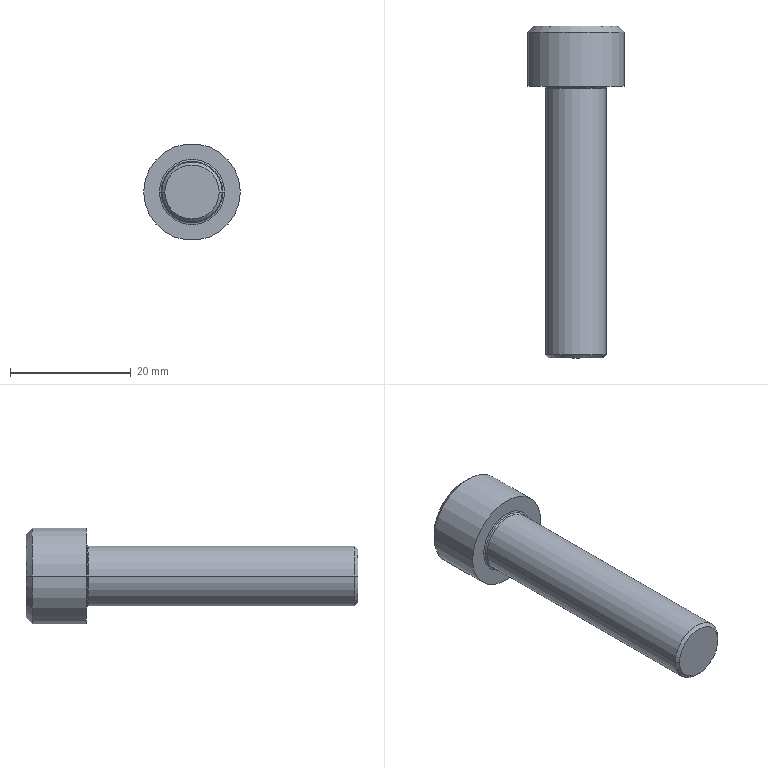Part | Creo | 1 solid | 23 faces | box 16 x 55 x 16 mm | volume 5183 mm3 | plane 9 | cone 6 | cylinder 4 | torus 4 | commonest cylinder face diameters 10 x2 16 x2
STEP:
#1=CARTESIAN_POINT('',(-18.457,360.995,-174.076));
#2=VERTEX_POINT('',#1);
#3=CARTESIAN_POINT('',(-20.767,360.995,-178.076));
#4=VERTEX_POINT('',#3);
#5=CARTESIAN_POINT('',(-18.457,360.995,-174.076));
#6=CARTESIAN_POINT('',(-18.565,360.933,-174.262));
#7=CARTESIAN_POINT('',(-18.781,360.821,-174.637));
#8=CARTESIAN_POINT('',(-19.11,360.7,-175.207));
#9=CARTESIAN_POINT('',(-19.444,360.635,-175.785));
#10=CARTESIAN_POINT('',(-19.779,360.635,-176.365));
#11=CARTESIAN_POINT('',(-20.113,360.7,-176.943));
#12=CARTESIAN_POINT('',(-20.442,360.821,-177.513));
#13=CARTESIAN_POINT('',(-20.659,360.933,-177.889));
#14=CARTESIAN_POINT('',(-20.767,360.995,-178.076));
#15=B_SPLINE_CURVE_WITH_KNOTS('',3,(#5,#6,#7,#8,#9,#10,#11,#12,#13,#14),.UNSPECIFIED.,.F.,.F.,(4,1,1,1,1,1,1,4),(0.,0.1429,0.2857,0.4286,0.5714,0.7143,0.8571,1.),.UNSPECIFIED.);
#16=EDGE_CURVE('',#2,#4,#15,.T.);
#17=ORIENTED_EDGE('',*,*,#16,.F.);
#18=CARTESIAN_POINT('',(-23.076,358.329,-174.076));
#19=VERTEX_POINT('',#18);
#20=CARTESIAN_POINT('',(-23.076,358.329,-174.076));
#21=DIRECTION('',(0.866,0.5,0.));
#22=VECTOR('',#21,5.333);
#23=LINE('',#20,#22);
#24=EDGE_CURVE('',#19,#2,#23,.T.);
#25=ORIENTED_EDGE('',*,*,#24,.F.);
#26=CARTESIAN_POINT('',(-27.695,360.995,-174.076));
#27=VERTEX_POINT('',#26);
#28=CARTESIAN_POINT('',(-23.076,358.329,-174.076));
#29=DIRECTION('',(-0.866,0.5,0.));
#30=VECTOR('',#29,5.333);
#31=LINE('',#28,#30);
#32=EDGE_CURVE('',#19,#27,#31,.T.);
#33=ORIENTED_EDGE('',*,*,#32,.T.);
#34=CARTESIAN_POINT('',(-25.386,360.995,-178.076));
#35=VERTEX_POINT('',#34);
#36=CARTESIAN_POINT('',(-25.386,360.995,-178.076));
#37=CARTESIAN_POINT('',(-25.493,360.933,-177.89));
#38=CARTESIAN_POINT('',(-25.709,360.821,-177.516));
#39=CARTESIAN_POINT('',(-26.039,360.7,-176.945));
#40=CARTESIAN_POINT('',(-26.372,360.635,-176.367));
#41=CARTESIAN_POINT('',(-26.707,360.635,-175.788));
#42=CARTESIAN_POINT('',(-27.041,360.7,-175.209));
#43=CARTESIAN_POINT('',(-27.37,360.821,-174.639));
#44=CARTESIAN_POINT('',(-27.587,360.933,-174.263));
#45=CARTESIAN_POINT('',(-27.695,360.995,-174.076));
#46=B_SPLINE_CURVE_WITH_KNOTS('',3,(#36,#37,#38,#39,#40,#41,#42,#43,#44,#45),.UNSPECIFIED.,.F.,.F.,(4,1,1,1,1,1,1,4),(0.,0.1429,0.2857,0.4286,0.5714,0.7143,0.8571,1.),.UNSPECIFIED.);
#47=EDGE_CURVE('',#35,#27,#46,.T.);
#48=ORIENTED_EDGE('',*,*,#47,.F.);
#49=CARTESIAN_POINT('',(-20.767,360.995,-178.076));
#50=CARTESIAN_POINT('',(-20.981,360.934,-178.076));
#51=CARTESIAN_POINT('',(-21.411,360.822,-178.076));
#52=CARTESIAN_POINT('',(-22.072,360.7,-178.076));
#53=CARTESIAN_POINT('',(-22.741,360.635,-178.076));
#54=CARTESIAN_POINT('',(-23.409,360.635,-178.076));
#55=CARTESIAN_POINT('',(-24.076,360.699,-178.076));
#56=CARTESIAN_POINT('',(-24.738,360.821,-178.076));
#57=CARTESIAN_POINT('',(-25.17,360.933,-178.076));
#58=CARTESIAN_POINT('',(-25.386,360.995,-178.076));
#59=B_SPLINE_CURVE_WITH_KNOTS('',3,(#49,#50,#51,#52,#53,#54,#55,#56,#57,#58),.UNSPECIFIED.,.F.,.F.,(4,1,1,1,1,1,1,4),(0.,0.1429,0.2857,0.4286,0.5714,0.7143,0.8571,1.),.UNSPECIFIED.);
#60=EDGE_CURVE('',#4,#35,#59,.T.);
#61=ORIENTED_EDGE('',*,*,#60,.F.);
#62=EDGE_LOOP('',(#17,#25,#33,#48,#61));
#63=FACE_OUTER_BOUND('',#62,.F.);
#64=CARTESIAN_POINT('',(-23.076,359.689,-174.076));
#65=DIRECTION('',(0.,1.,0.));
#66=DIRECTION('',(1.,0.,0.));
#67=AXIS2_PLACEMENT_3D('',#64,#65,#66);
#68=CONICAL_SURFACE('',#67,2.356,60.);
#69=ADVANCED_FACE('',(#63),#68,.F.);
#70=CARTESIAN_POINT('',(-20.767,365.995,-178.076));
#71=VERTEX_POINT('',#70);
#72=CARTESIAN_POINT('',(-18.457,365.995,-174.076));
#73=VERTEX_POINT('',#72);
#74=CARTESIAN_POINT('',(-20.767,365.995,-178.076));
#75=DIRECTION('',(0.5,0.,0.866));
#76=VECTOR('',#75,4.619);
#77=LINE('',#74,#76);
#78=EDGE_CURVE('',#71,#73,#77,.T.);
#79=ORIENTED_EDGE('',*,*,#78,.T.);
#80=CARTESIAN_POINT('',(-18.457,365.995,-174.076));
#81=DIRECTION('',(0.,-1.,0.));
#82=VECTOR('',#81,5.);
#83=LINE('',#80,#82);
#84=EDGE_CURVE('',#73,#2,#83,.T.);
#85=ORIENTED_EDGE('',*,*,#84,.T.);
#86=ORIENTED_EDGE('',*,*,#16,.T.);
#87=CARTESIAN_POINT('',(-20.767,365.995,-178.076));
#88=DIRECTION('',(0.,-1.,0.));
#89=VECTOR('',#88,5.);
#90=LINE('',#87,#89);
#91=EDGE_CURVE('',#71,#4,#90,.T.);
#92=ORIENTED_EDGE('',*,*,#91,.F.);
#93=EDGE_LOOP('',(#79,#85,#86,#92));
#94=FACE_OUTER_BOUND('',#93,.F.);
#95=CARTESIAN_POINT('',(-20.767,360.995,-178.076));
#96=DIRECTION('',(-0.866,0.,0.5));
#97=DIRECTION('',(0.5,0.,0.866));
#98=AXIS2_PLACEMENT_3D('',#95,#96,#97);
#99=PLANE('',#98);
#100=ADVANCED_FACE('',(#94),#99,.T.);
#101=CARTESIAN_POINT('',(-16.076,365.995,-174.076));
#102=VERTEX_POINT('',#101);
#103=CARTESIAN_POINT('',(-30.076,365.995,-174.076));
#104=VERTEX_POINT('',#103);
#105=CARTESIAN_POINT('',(-23.076,365.995,-174.076));
#106=DIRECTION('',(0.,1.,0.));
#107=DIRECTION('',(1.,0.,0.));
#108=AXIS2_PLACEMENT_3D('',#105,#106,#107);
#109=CIRCLE('',#108,7.);
#110=EDGE_CURVE('',#102,#104,#109,.T.);
#111=ORIENTED_EDGE('',*,*,#110,.F.);
#112=CARTESIAN_POINT('',(-23.076,365.995,-174.076));
#113=DIRECTION('',(0.,1.,0.));
#114=DIRECTION('',(-1.,0.,0.));
#115=AXIS2_PLACEMENT_3D('',#112,#113,#114);
#116=CIRCLE('',#115,7.);
#117=EDGE_CURVE('',#104,#102,#116,.T.);
#118=ORIENTED_EDGE('',*,*,#117,.F.);
#119=EDGE_LOOP('',(#111,#118));
#120=FACE_OUTER_BOUND('',#119,.F.);
#121=CARTESIAN_POINT('',(-20.767,365.995,-170.076));
#122=VERTEX_POINT('',#121);
#123=CARTESIAN_POINT('',(-18.457,365.995,-174.076));
#124=DIRECTION('',(-0.5,0.,0.866));
#125=VECTOR('',#124,4.619);
#126=LINE('',#123,#125);
#127=EDGE_CURVE('',#73,#122,#126,.T.);
#128=ORIENTED_EDGE('',*,*,#127,.F.);
#129=ORIENTED_EDGE('',*,*,#78,.F.);
#130=CARTESIAN_POINT('',(-25.386,365.995,-178.076));
#131=VERTEX_POINT('',#130);
#132=CARTESIAN_POINT('',(-20.767,365.995,-178.076));
#133=DIRECTION('',(-1.,0.,0.));
#134=VECTOR('',#133,4.619);
#135=LINE('',#132,#134);
#136=EDGE_CURVE('',#71,#131,#135,.T.);
#137=ORIENTED_EDGE('',*,*,#136,.T.);
#138=CARTESIAN_POINT('',(-27.695,365.995,-174.076));
#139=VERTEX_POINT('',#138);
#140=CARTESIAN_POINT('',(-27.695,365.995,-174.076));
#141=DIRECTION('',(0.5,0.,-0.866));
#142=VECTOR('',#141,4.619);
#143=LINE('',#140,#142);
#144=EDGE_CURVE('',#139,#131,#143,.T.);
#145=ORIENTED_EDGE('',*,*,#144,.F.);
#146=CARTESIAN_POINT('',(-25.386,365.995,-170.076));
#147=VERTEX_POINT('',#146);
#148=CARTESIAN_POINT('',(-25.386,365.995,-170.076));
#149=DIRECTION('',(-0.5,0.,-0.866));
#150=VECTOR('',#149,4.619);
#151=LINE('',#148,#150);
#152=EDGE_CURVE('',#147,#139,#151,.T.);
#153=ORIENTED_EDGE('',*,*,#152,.F.);
#154=CARTESIAN_POINT('',(-25.386,365.995,-170.076));
#155=DIRECTION('',(1.,0.,0.));
#156=VECTOR('',#155,4.619);
#157=LINE('',#154,#156);
#158=EDGE_CURVE('',#147,#122,#157,.T.);
#159=ORIENTED_EDGE('',*,*,#158,.T.);
#160=EDGE_LOOP('',(#128,#129,#137,#145,#153,#159));
#161=FACE_BOUND('',#160,.F.);
#162=CARTESIAN_POINT('',(-23.076,365.995,-174.076));
#163=DIRECTION('',(0.,1.,0.));
#164=DIRECTION('',(1.,0.,0.));
#165=AXIS2_PLACEMENT_3D('',#162,#163,#164);
#166=PLANE('',#165);
#167=ADVANCED_FACE('',(#120,#161),#166,.T.);
#168=CARTESIAN_POINT('',(-15.076,364.995,-174.076));
#169=VERTEX_POINT('',#168);
#170=CARTESIAN_POINT('',(-31.076,364.995,-174.076));
#171=VERTEX_POINT('',#170);
#172=CARTESIAN_POINT('',(-23.076,364.995,-174.076));
#173=DIRECTION('',(0.,1.,0.));
#174=DIRECTION('',(1.,0.,0.));
#175=AXIS2_PLACEMENT_3D('',#172,#173,#174);
#176=CIRCLE('',#175,8.);
#177=EDGE_CURVE('',#169,#171,#176,.T.);
#178=ORIENTED_EDGE('',*,*,#177,.F.);
#179=CARTESIAN_POINT('',(-16.076,365.995,-174.076));
#180=DIRECTION('',(0.7071,-0.7071,0.));
#181=VECTOR('',#180,1.414);
#182=LINE('',#179,#181);
#183=EDGE_CURVE('',#102,#169,#182,.T.);
#184=ORIENTED_EDGE('',*,*,#183,.F.);
#185=ORIENTED_EDGE('',*,*,#110,.T.);
#186=CARTESIAN_POINT('',(-30.076,365.995,-174.076));
#187=DIRECTION('',(-0.7071,-0.7071,0.));
#188=VECTOR('',#187,1.414);
#189=LINE('',#186,#188);
#190=EDGE_CURVE('',#104,#171,#189,.T.);
#191=ORIENTED_EDGE('',*,*,#190,.T.);
#192=EDGE_LOOP('',(#178,#184,#185,#191));
#193=FACE_OUTER_BOUND('',#192,.F.);
#194=CARTESIAN_POINT('',(-23.076,365.495,-174.076));
#195=DIRECTION('',(0.,-1.,0.));
#196=DIRECTION('',(-1.,0.,0.));
#197=AXIS2_PLACEMENT_3D('',#194,#195,#196);
#198=CONICAL_SURFACE('',#197,7.5,45.);
#199=ADVANCED_FACE('',(#193),#198,.T.);
#200=ORIENTED_EDGE('',*,*,#177,.T.);
#201=CARTESIAN_POINT('',(-31.076,355.995,-174.076));
#202=VERTEX_POINT('',#201);
#203=CARTESIAN_POINT('',(-31.076,355.995,-174.076));
#204=DIRECTION('',(0.,1.,0.));
#205=VECTOR('',#204,9.);
#206=LINE('',#203,#205);
#207=EDGE_CURVE('',#202,#171,#206,.T.);
#208=ORIENTED_EDGE('',*,*,#207,.F.);
#209=CARTESIAN_POINT('',(-15.076,355.995,-174.076));
#210=VERTEX_POINT('',#209);
#211=CARTESIAN_POINT('',(-23.076,355.995,-174.076));
#212=DIRECTION('',(0.,-1.,0.));
#213=DIRECTION('',(-1.,0.,0.));
#214=AXIS2_PLACEMENT_3D('',#211,#212,#213);
#215=CIRCLE('',#214,8.);
#216=EDGE_CURVE('',#202,#210,#215,.T.);
#217=ORIENTED_EDGE('',*,*,#216,.T.);
#218=CARTESIAN_POINT('',(-15.076,355.995,-174.076));
#219=DIRECTION('',(0.,1.,0.));
#220=VECTOR('',#219,9.);
#221=LINE('',#218,#220);
#222=EDGE_CURVE('',#210,#169,#221,.T.);
#223=ORIENTED_EDGE('',*,*,#222,.T.);
#224=EDGE_LOOP('',(#200,#208,#217,#223));
#225=FACE_OUTER_BOUND('',#224,.F.);
#226=CARTESIAN_POINT('',(-23.076,355.995,-174.076));
#227=DIRECTION('',(0.,1.,0.));
#228=DIRECTION('',(1.,0.,0.));
#229=AXIS2_PLACEMENT_3D('',#226,#227,#228);
#230=CYLINDRICAL_SURFACE('',#229,8.);
#231=ADVANCED_FACE('',(#225),#230,.T.);
#232=CARTESIAN_POINT('',(-23.076,364.995,-174.076));
#233=DIRECTION('',(0.,1.,0.));
#234=DIRECTION('',(-1.,0.,0.));
#235=AXIS2_PLACEMENT_3D('',#232,#233,#234);
#236=CIRCLE('',#235,8.);
#237=EDGE_CURVE('',#171,#169,#236,.T.);
#238=ORIENTED_EDGE('',*,*,#237,.T.);
#239=ORIENTED_EDGE('',*,*,#222,.F.);
#240=CARTESIAN_POINT('',(-23.076,355.995,-174.076));
#241=DIRECTION('',(0.,-1.,0.));
#242=DIRECTION('',(1.,0.,0.));
#243=AXIS2_PLACEMENT_3D('',#240,#241,#242);
#244=CIRCLE('',#243,8.);
#245=EDGE_CURVE('',#210,#202,#244,.T.);
#246=ORIENTED_EDGE('',*,*,#245,.T.);
#247=ORIENTED_EDGE('',*,*,#207,.T.);
#248=EDGE_LOOP('',(#238,#239,#246,#247));
#249=FACE_OUTER_BOUND('',#248,.F.);
#250=CARTESIAN_POINT('',(-23.076,355.995,-174.076));
#251=DIRECTION('',(0.,1.,0.));
#252=DIRECTION('',(1.,0.,0.));
#253=AXIS2_PLACEMENT_3D('',#250,#251,#252);
#254=CYLINDRICAL_SURFACE('',#253,8.);
#255=ADVANCED_FACE('',(#249),#254,.T.);
#256=ORIENTED_EDGE('',*,*,#237,.F.);
#257=ORIENTED_EDGE('',*,*,#190,.F.);
#258=ORIENTED_EDGE('',*,*,#117,.T.);
#259=ORIENTED_EDGE('',*,*,#183,.T.);
#260=EDGE_LOOP('',(#256,#257,#258,#259));
#261=FACE_OUTER_BOUND('',#260,.F.);
#262=CARTESIAN_POINT('',(-23.076,365.495,-174.076));
#263=DIRECTION('',(0.,-1.,0.));
#264=DIRECTION('',(-1.,0.,0.));
#265=AXIS2_PLACEMENT_3D('',#262,#263,#264);
#266=CONICAL_SURFACE('',#265,7.5,45.);
#267=ADVANCED_FACE('',(#261),#266,.T.);
#268=ORIENTED_EDGE('',*,*,#245,.F.);
#269=ORIENTED_EDGE('',*,*,#216,.F.);
#270=EDGE_LOOP('',(#268,#269));
#271=FACE_OUTER_BOUND('',#270,.F.);
#272=CARTESIAN_POINT('',(-17.676,355.995,-174.076));
#273=VERTEX_POINT('',#272);
#274=CARTESIAN_POINT('',(-28.476,355.995,-174.076));
#275=VERTEX_POINT('',#274);
#276=CARTESIAN_POINT('',(-23.076,355.995,-174.076));
#277=DIRECTION('',(0.,1.,0.));
#278=DIRECTION('',(1.,0.,0.));
#279=AXIS2_PLACEMENT_3D('',#276,#277,#278);
#280=CIRCLE('',#279,5.4);
#281=EDGE_CURVE('',#273,#275,#280,.T.);
#282=ORIENTED_EDGE('',*,*,#281,.F.);
#283=CARTESIAN_POINT('',(-23.076,355.995,-174.076));
#284=DIRECTION('',(0.,1.,0.));
#285=DIRECTION('',(-1.,0.,0.));
#286=AXIS2_PLACEMENT_3D('',#283,#284,#285);
#287=CIRCLE('',#286,5.4);
#288=EDGE_CURVE('',#275,#273,#287,.T.);
#289=ORIENTED_EDGE('',*,*,#288,.F.);
#290=EDGE_LOOP('',(#282,#289));
#291=FACE_BOUND('',#290,.F.);
#292=CARTESIAN_POINT('',(-23.076,355.995,-174.076));
#293=DIRECTION('',(0.,1.,0.));
#294=DIRECTION('',(1.,0.,0.));
#295=AXIS2_PLACEMENT_3D('',#292,#293,#294);
#296=PLANE('',#295);
#297=ADVANCED_FACE('',(#271,#291),#296,.F.);
#298=ORIENTED_EDGE('',*,*,#281,.T.);
#299=CARTESIAN_POINT('',(-28.193,355.878,-174.076));
#300=VERTEX_POINT('',#299);
#301=CARTESIAN_POINT('',(-28.476,355.595,-174.076));
#302=DIRECTION('',(0.,0.,-1.));
#303=DIRECTION('',(0.,1.,0.));
#304=AXIS2_PLACEMENT_3D('',#301,#302,#303);
#305=CIRCLE('',#304,0.4);
#306=EDGE_CURVE('',#275,#300,#305,.T.);
#307=ORIENTED_EDGE('',*,*,#306,.T.);
#308=CARTESIAN_POINT('',(-17.959,355.878,-174.076));
#309=VERTEX_POINT('',#308);
#310=CARTESIAN_POINT('',(-23.076,355.878,-174.076));
#311=DIRECTION('',(0.,1.,0.));
#312=DIRECTION('',(1.,0.,0.));
#313=AXIS2_PLACEMENT_3D('',#310,#311,#312);
#314=CIRCLE('',#313,5.117);
#315=EDGE_CURVE('',#309,#300,#314,.T.);
#316=ORIENTED_EDGE('',*,*,#315,.F.);
#317=CARTESIAN_POINT('',(-17.676,355.595,-174.076));
#318=DIRECTION('',(0.,0.,1.));
#319=DIRECTION('',(0.,1.,0.));
#320=AXIS2_PLACEMENT_3D('',#317,#318,#319);
#321=CIRCLE('',#320,0.4);
#322=EDGE_CURVE('',#273,#309,#321,.T.);
#323=ORIENTED_EDGE('',*,*,#322,.F.);
#324=EDGE_LOOP('',(#298,#307,#316,#323));
#325=FACE_OUTER_BOUND('',#324,.F.);
#326=CARTESIAN_POINT('',(-23.076,355.595,-174.076));
#327=DIRECTION('',(0.,1.,0.));
#328=DIRECTION('',(1.,0.,0.));
#329=AXIS2_PLACEMENT_3D('',#326,#327,#328);
#330=TOROIDAL_SURFACE('',#329,5.4,0.4);
#331=ADVANCED_FACE('',(#325),#330,.F.);
#332=ORIENTED_EDGE('',*,*,#288,.T.);
#333=ORIENTED_EDGE('',*,*,#322,.T.);
#334=CARTESIAN_POINT('',(-23.076,355.878,-174.076));
#335=DIRECTION('',(0.,1.,0.));
#336=DIRECTION('',(-1.,0.,0.));
#337=AXIS2_PLACEMENT_3D('',#334,#335,#336);
#338=CIRCLE('',#337,5.117);
#339=EDGE_CURVE('',#300,#309,#338,.T.);
#340=ORIENTED_EDGE('',*,*,#339,.F.);
#341=ORIENTED_EDGE('',*,*,#306,.F.);
#342=EDGE_LOOP('',(#332,#333,#340,#341));
#343=FACE_OUTER_BOUND('',#342,.F.);
#344=CARTESIAN_POINT('',(-23.076,355.595,-174.076));
#345=DIRECTION('',(0.,1.,0.));
#346=DIRECTION('',(1.,0.,0.));
#347=AXIS2_PLACEMENT_3D('',#344,#345,#346);
#348=TOROIDAL_SURFACE('',#347,5.4,0.4);
#349=ADVANCED_FACE('',(#343),#348,.F.);
#350=CARTESIAN_POINT('',(-28.076,355.595,-174.076));
#351=VERTEX_POINT('',#350);
#352=CARTESIAN_POINT('',(-18.076,355.595,-174.076));
#353=VERTEX_POINT('',#352);
#354=CARTESIAN_POINT('',(-23.076,355.595,-174.076));
#355=DIRECTION('',(0.,1.,0.));
#356=DIRECTION('',(-1.,0.,0.));
#357=AXIS2_PLACEMENT_3D('',#354,#355,#356);
#358=CIRCLE('',#357,5.);
#359=EDGE_CURVE('',#351,#353,#358,.T.);
#360=ORIENTED_EDGE('',*,*,#359,.F.);
#361=CARTESIAN_POINT('',(-28.476,355.595,-174.076));
#362=DIRECTION('',(0.,0.,-1.));
#363=DIRECTION('',(0.7071,0.7071,0.));
#364=AXIS2_PLACEMENT_3D('',#361,#362,#363);
#365=CIRCLE('',#364,0.4);
#366=EDGE_CURVE('',#300,#351,#365,.T.);
#367=ORIENTED_EDGE('',*,*,#366,.F.);
#368=ORIENTED_EDGE('',*,*,#339,.T.);
#369=CARTESIAN_POINT('',(-17.676,355.595,-174.076));
#370=DIRECTION('',(0.,0.,1.));
#371=DIRECTION('',(-0.7071,0.7071,0.));
#372=AXIS2_PLACEMENT_3D('',#369,#370,#371);
#373=CIRCLE('',#372,0.4);
#374=EDGE_CURVE('',#309,#353,#373,.T.);
#375=ORIENTED_EDGE('',*,*,#374,.T.);
#376=EDGE_LOOP('',(#360,#367,#368,#375));
#377=FACE_OUTER_BOUND('',#376,.F.);
#378=CARTESIAN_POINT('',(-23.076,355.595,-174.076));
#379=DIRECTION('',(0.,1.,0.));
#380=DIRECTION('',(1.,0.,0.));
#381=AXIS2_PLACEMENT_3D('',#378,#379,#380);
#382=TOROIDAL_SURFACE('',#381,5.4,0.4);
#383=ADVANCED_FACE('',(#377),#382,.F.);
#384=CARTESIAN_POINT('',(-18.076,311.495,-174.076));
#385=VERTEX_POINT('',#384);
#386=CARTESIAN_POINT('',(-28.076,311.495,-174.076));
#387=VERTEX_POINT('',#386);
#388=CARTESIAN_POINT('',(-23.076,311.495,-174.076));
#389=DIRECTION('',(0.,-1.,0.));
#390=DIRECTION('',(1.,0.,0.));
#391=AXIS2_PLACEMENT_3D('',#388,#389,#390);
#392=CIRCLE('',#391,5.);
#393=EDGE_CURVE('',#385,#387,#392,.T.);
#394=ORIENTED_EDGE('',*,*,#393,.T.);
#395=CARTESIAN_POINT('',(-28.076,311.495,-174.076));
#396=DIRECTION('',(0.,1.,0.));
#397=VECTOR('',#396,44.1);
#398=LINE('',#395,#397);
#399=EDGE_CURVE('',#387,#351,#398,.T.);
#400=ORIENTED_EDGE('',*,*,#399,.T.);
#401=ORIENTED_EDGE('',*,*,#359,.T.);
#402=CARTESIAN_POINT('',(-18.076,311.495,-174.076));
#403=DIRECTION('',(0.,1.,0.));
#404=VECTOR('',#403,44.1);
#405=LINE('',#402,#404);
#406=EDGE_CURVE('',#385,#353,#405,.T.);
#407=ORIENTED_EDGE('',*,*,#406,.F.);
#408=EDGE_LOOP('',(#394,#400,#401,#407));
#409=FACE_OUTER_BOUND('',#408,.F.);
#410=CARTESIAN_POINT('',(-23.076,310.995,-174.076));
#411=DIRECTION('',(0.,1.,0.));
#412=DIRECTION('',(1.,0.,0.));
#413=AXIS2_PLACEMENT_3D('',#410,#411,#412);
#414=CYLINDRICAL_SURFACE('',#413,5.);
#415=ADVANCED_FACE('',(#409),#414,.T.);
#416=CARTESIAN_POINT('',(-18.576,310.995,-174.076));
#417=VERTEX_POINT('',#416);
#418=CARTESIAN_POINT('',(-27.576,310.995,-174.076));
#419=VERTEX_POINT('',#418);
#420=CARTESIAN_POINT('',(-23.076,310.995,-174.076));
#421=DIRECTION('',(0.,-1.,0.));
#422=DIRECTION('',(1.,0.,0.));
#423=AXIS2_PLACEMENT_3D('',#420,#421,#422);
#424=CIRCLE('',#423,4.5);
#425=EDGE_CURVE('',#417,#419,#424,.T.);
#426=ORIENTED_EDGE('',*,*,#425,.T.);
#427=CARTESIAN_POINT('',(-27.576,310.995,-174.076));
#428=DIRECTION('',(-0.7071,0.7071,0.));
#429=VECTOR('',#428,0.7071);
#430=LINE('',#427,#429);
#431=EDGE_CURVE('',#419,#387,#430,.T.);
#432=ORIENTED_EDGE('',*,*,#431,.T.);
#433=ORIENTED_EDGE('',*,*,#393,.F.);
#434=CARTESIAN_POINT('',(-18.576,310.995,-174.076));
#435=DIRECTION('',(0.7071,0.7071,0.));
#436=VECTOR('',#435,0.7071);
#437=LINE('',#434,#436);
#438=EDGE_CURVE('',#417,#385,#437,.T.);
#439=ORIENTED_EDGE('',*,*,#438,.F.);
#440=EDGE_LOOP('',(#426,#432,#433,#439));
#441=FACE_OUTER_BOUND('',#440,.F.);
#442=CARTESIAN_POINT('',(-23.076,311.245,-174.076));
#443=DIRECTION('',(0.,1.,0.));
#444=DIRECTION('',(1.,0.,0.));
#445=AXIS2_PLACEMENT_3D('',#442,#443,#444);
#446=CONICAL_SURFACE('',#445,4.75,45.);
#447=ADVANCED_FACE('',(#441),#446,.T.);
#448=ORIENTED_EDGE('',*,*,#425,.F.);
#449=CARTESIAN_POINT('',(-23.076,310.995,-174.076));
#450=DIRECTION('',(0.,-1.,0.));
#451=DIRECTION('',(-1.,0.,0.));
#452=AXIS2_PLACEMENT_3D('',#449,#450,#451);
#453=CIRCLE('',#452,4.5);
#454=EDGE_CURVE('',#419,#417,#453,.T.);
#455=ORIENTED_EDGE('',*,*,#454,.F.);
#456=EDGE_LOOP('',(#448,#455));
#457=FACE_OUTER_BOUND('',#456,.F.);
#458=CARTESIAN_POINT('',(-23.076,310.995,-174.076));
#459=DIRECTION('',(0.,1.,0.));
#460=DIRECTION('',(1.,0.,0.));
#461=AXIS2_PLACEMENT_3D('',#458,#459,#460);
#462=PLANE('',#461);
#463=ADVANCED_FACE('',(#457),#462,.F.);
#464=ORIENTED_EDGE('',*,*,#454,.T.);
#465=ORIENTED_EDGE('',*,*,#438,.T.);
#466=CARTESIAN_POINT('',(-23.076,311.495,-174.076));
#467=DIRECTION('',(0.,-1.,0.));
#468=DIRECTION('',(-1.,0.,0.));
#469=AXIS2_PLACEMENT_3D('',#466,#467,#468);
#470=CIRCLE('',#469,5.);
#471=EDGE_CURVE('',#387,#385,#470,.T.);
#472=ORIENTED_EDGE('',*,*,#471,.F.);
#473=ORIENTED_EDGE('',*,*,#431,.F.);
#474=EDGE_LOOP('',(#464,#465,#472,#473));
#475=FACE_OUTER_BOUND('',#474,.F.);
#476=CARTESIAN_POINT('',(-23.076,311.245,-174.076));
#477=DIRECTION('',(0.,1.,0.));
#478=DIRECTION('',(1.,0.,0.));
#479=AXIS2_PLACEMENT_3D('',#476,#477,#478);
#480=CONICAL_SURFACE('',#479,4.75,45.);
#481=ADVANCED_FACE('',(#475),#480,.T.);
#482=ORIENTED_EDGE('',*,*,#471,.T.);
#483=ORIENTED_EDGE('',*,*,#406,.T.);
#484=CARTESIAN_POINT('',(-23.076,355.595,-174.076));
#485=DIRECTION('',(0.,1.,0.));
#486=DIRECTION('',(1.,0.,0.));
#487=AXIS2_PLACEMENT_3D('',#484,#485,#486);
#488=CIRCLE('',#487,5.);
#489=EDGE_CURVE('',#353,#351,#488,.T.);
#490=ORIENTED_EDGE('',*,*,#489,.T.);
#491=ORIENTED_EDGE('',*,*,#399,.F.);
#492=EDGE_LOOP('',(#482,#483,#490,#491));
#493=FACE_OUTER_BOUND('',#492,.F.);
#494=CARTESIAN_POINT('',(-23.076,310.995,-174.076));
#495=DIRECTION('',(0.,1.,0.));
#496=DIRECTION('',(1.,0.,0.));
#497=AXIS2_PLACEMENT_3D('',#494,#495,#496);
#498=CYLINDRICAL_SURFACE('',#497,5.);
#499=ADVANCED_FACE('',(#493),#498,.T.);
#500=ORIENTED_EDGE('',*,*,#489,.F.);
#501=ORIENTED_EDGE('',*,*,#374,.F.);
#502=ORIENTED_EDGE('',*,*,#315,.T.);
#503=ORIENTED_EDGE('',*,*,#366,.T.);
#504=EDGE_LOOP('',(#500,#501,#502,#503));
#505=FACE_OUTER_BOUND('',#504,.F.);
#506=CARTESIAN_POINT('',(-23.076,355.595,-174.076));
#507=DIRECTION('',(0.,1.,0.));
#508=DIRECTION('',(1.,0.,0.));
#509=AXIS2_PLACEMENT_3D('',#506,#507,#508);
#510=TOROIDAL_SURFACE('',#509,5.4,0.4);
#511=ADVANCED_FACE('',(#505),#510,.F.);
#512=ORIENTED_EDGE('',*,*,#127,.T.);
#513=CARTESIAN_POINT('',(-20.767,360.995,-170.076));
#514=VERTEX_POINT('',#513);
#515=CARTESIAN_POINT('',(-20.767,365.995,-170.076));
#516=DIRECTION('',(0.,-1.,0.));
#517=VECTOR('',#516,5.);
#518=LINE('',#515,#517);
#519=EDGE_CURVE('',#122,#514,#518,.T.);
#520=ORIENTED_EDGE('',*,*,#519,.T.);
#521=CARTESIAN_POINT('',(-20.767,360.995,-170.076));
#522=CARTESIAN_POINT('',(-20.659,360.933,-170.262));
#523=CARTESIAN_POINT('',(-20.443,360.821,-170.637));
#524=CARTESIAN_POINT('',(-20.114,360.7,-171.207));
#525=CARTESIAN_POINT('',(-19.78,360.635,-171.785));
#526=CARTESIAN_POINT('',(-19.446,360.635,-172.365));
#527=CARTESIAN_POINT('',(-19.112,360.7,-172.943));
#528=CARTESIAN_POINT('',(-18.782,360.821,-173.513));
#529=CARTESIAN_POINT('',(-18.565,360.933,-173.889));
#530=CARTESIAN_POINT('',(-18.457,360.995,-174.076));
#531=B_SPLINE_CURVE_WITH_KNOTS('',3,(#521,#522,#523,#524,#525,#526,#527,#528,#529,#530),.UNSPECIFIED.,.F.,.F.,(4,1,1,1,1,1,1,4),(0.,0.1429,0.2857,0.4286,0.5714,0.7143,0.8571,1.),.UNSPECIFIED.);
#532=EDGE_CURVE('',#514,#2,#531,.T.);
#533=ORIENTED_EDGE('',*,*,#532,.T.);
#534=ORIENTED_EDGE('',*,*,#84,.F.);
#535=EDGE_LOOP('',(#512,#520,#533,#534));
#536=FACE_OUTER_BOUND('',#535,.F.);
#537=CARTESIAN_POINT('',(-18.457,360.995,-174.076));
#538=DIRECTION('',(-0.866,0.,-0.5));
#539=DIRECTION('',(-0.5,0.,0.866));
#540=AXIS2_PLACEMENT_3D('',#537,#538,#539);
#541=PLANE('',#540);
#542=ADVANCED_FACE('',(#536),#541,.T.);
#543=ORIENTED_EDGE('',*,*,#158,.F.);
#544=CARTESIAN_POINT('',(-25.386,360.995,-170.076));
#545=VERTEX_POINT('',#544);
#546=CARTESIAN_POINT('',(-25.386,365.995,-170.076));
#547=DIRECTION('',(0.,-1.,0.));
#548=VECTOR('',#547,5.);
#549=LINE('',#546,#548);
#550=EDGE_CURVE('',#147,#545,#549,.T.);
#551=ORIENTED_EDGE('',*,*,#550,.T.);
#552=CARTESIAN_POINT('',(-25.386,360.995,-170.076));
#553=CARTESIAN_POINT('',(-25.17,360.933,-170.076));
#554=CARTESIAN_POINT('',(-24.738,360.821,-170.076));
#555=CARTESIAN_POINT('',(-24.076,360.699,-170.076));
#556=CARTESIAN_POINT('',(-23.409,360.635,-170.076));
#557=CARTESIAN_POINT('',(-22.741,360.635,-170.076));
#558=CARTESIAN_POINT('',(-22.072,360.7,-170.076));
#559=CARTESIAN_POINT('',(-21.411,360.822,-170.076));
#560=CARTESIAN_POINT('',(-20.981,360.934,-170.076));
#561=CARTESIAN_POINT('',(-20.767,360.995,-170.076));
#562=B_SPLINE_CURVE_WITH_KNOTS('',3,(#552,#553,#554,#555,#556,#557,#558,#559,#560,#561),.UNSPECIFIED.,.F.,.F.,(4,1,1,1,1,1,1,4),(0.,0.1429,0.2857,0.4286,0.5714,0.7143,0.8571,1.),.UNSPECIFIED.);
#563=EDGE_CURVE('',#545,#514,#562,.T.);
#564=ORIENTED_EDGE('',*,*,#563,.T.);
#565=ORIENTED_EDGE('',*,*,#519,.F.);
#566=EDGE_LOOP('',(#543,#551,#564,#565));
#567=FACE_OUTER_BOUND('',#566,.F.);
#568=CARTESIAN_POINT('',(-20.767,360.995,-170.076));
#569=DIRECTION('',(0.,0.,-1.));
#570=DIRECTION('',(0.,1.,0.));
#571=AXIS2_PLACEMENT_3D('',#568,#569,#570);
#572=PLANE('',#571);
#573=ADVANCED_FACE('',(#567),#572,.T.);
#574=ORIENTED_EDGE('',*,*,#152,.T.);
#575=CARTESIAN_POINT('',(-27.695,365.995,-174.076));
#576=DIRECTION('',(0.,-1.,0.));
#577=VECTOR('',#576,5.);
#578=LINE('',#575,#577);
#579=EDGE_CURVE('',#139,#27,#578,.T.);
#580=ORIENTED_EDGE('',*,*,#579,.T.);
#581=CARTESIAN_POINT('',(-27.695,360.995,-174.076));
#582=CARTESIAN_POINT('',(-27.587,360.933,-173.889));
#583=CARTESIAN_POINT('',(-27.37,360.821,-173.513));
#584=CARTESIAN_POINT('',(-27.041,360.7,-172.943));
#585=CARTESIAN_POINT('',(-26.707,360.635,-172.365));
#586=CARTESIAN_POINT('',(-26.372,360.635,-171.785));
#587=CARTESIAN_POINT('',(-26.039,360.7,-171.207));
#588=CARTESIAN_POINT('',(-25.709,360.821,-170.637));
#589=CARTESIAN_POINT('',(-25.493,360.933,-170.262));
#590=CARTESIAN_POINT('',(-25.386,360.995,-170.076));
#591=B_SPLINE_CURVE_WITH_KNOTS('',3,(#581,#582,#583,#584,#585,#586,#587,#588,#589,#590),.UNSPECIFIED.,.F.,.F.,(4,1,1,1,1,1,1,4),(0.,0.1429,0.2857,0.4286,0.5714,0.7143,0.8571,1.),.UNSPECIFIED.);
#592=EDGE_CURVE('',#27,#545,#591,.T.);
#593=ORIENTED_EDGE('',*,*,#592,.T.);
#594=ORIENTED_EDGE('',*,*,#550,.F.);
#595=EDGE_LOOP('',(#574,#580,#593,#594));
#596=FACE_OUTER_BOUND('',#595,.F.);
#597=CARTESIAN_POINT('',(-25.386,360.995,-170.076));
#598=DIRECTION('',(0.866,0.,-0.5));
#599=DIRECTION('',(-0.5,0.,-0.866));
#600=AXIS2_PLACEMENT_3D('',#597,#598,#599);
#601=PLANE('',#600);
#602=ADVANCED_FACE('',(#596),#601,.T.);
#603=ORIENTED_EDGE('',*,*,#144,.T.);
#604=CARTESIAN_POINT('',(-25.386,365.995,-178.076));
#605=DIRECTION('',(0.,-1.,0.));
#606=VECTOR('',#605,5.);
#607=LINE('',#604,#606);
#608=EDGE_CURVE('',#131,#35,#607,.T.);
#609=ORIENTED_EDGE('',*,*,#608,.T.);
#610=ORIENTED_EDGE('',*,*,#47,.T.);
#611=ORIENTED_EDGE('',*,*,#579,.F.);
#612=EDGE_LOOP('',(#603,#609,#610,#611));
#613=FACE_OUTER_BOUND('',#612,.F.);
#614=CARTESIAN_POINT('',(-27.695,360.995,-174.076));
#615=DIRECTION('',(0.866,0.,0.5));
#616=DIRECTION('',(0.5,0.,-0.866));
#617=AXIS2_PLACEMENT_3D('',#614,#615,#616);
#618=PLANE('',#617);
#619=ADVANCED_FACE('',(#613),#618,.T.);
#620=ORIENTED_EDGE('',*,*,#136,.F.);
#621=ORIENTED_EDGE('',*,*,#91,.T.);
#622=ORIENTED_EDGE('',*,*,#60,.T.);
#623=ORIENTED_EDGE('',*,*,#608,.F.);
#624=EDGE_LOOP('',(#620,#621,#622,#623));
#625=FACE_OUTER_BOUND('',#624,.F.);
#626=CARTESIAN_POINT('',(-25.386,360.995,-178.076));
#627=DIRECTION('',(0.,0.,1.));
#628=DIRECTION('',(0.,-1.,0.));
#629=AXIS2_PLACEMENT_3D('',#626,#627,#628);
#630=PLANE('',#629);
#631=ADVANCED_FACE('',(#625),#630,.T.);
#632=ORIENTED_EDGE('',*,*,#592,.F.);
#633=ORIENTED_EDGE('',*,*,#32,.F.);
#634=ORIENTED_EDGE('',*,*,#24,.T.);
#635=ORIENTED_EDGE('',*,*,#532,.F.);
#636=ORIENTED_EDGE('',*,*,#563,.F.);
#637=EDGE_LOOP('',(#632,#633,#634,#635,#636));
#638=FACE_OUTER_BOUND('',#637,.F.);
#639=CARTESIAN_POINT('',(-23.076,359.689,-174.076));
#640=DIRECTION('',(0.,1.,0.));
#641=DIRECTION('',(1.,0.,0.));
#642=AXIS2_PLACEMENT_3D('',#639,#640,#641);
#643=CONICAL_SURFACE('',#642,2.356,60.);
#644=ADVANCED_FACE('',(#638),#643,.F.);
#645=CLOSED_SHELL('',(#69,#100,#167,#199,#231,#255,#267,#297,#331,#349,#383,#415,#447,#463,#481,#499,#511,#542,#573,#602,#619,#631,#644));
#646=MANIFOLD_SOLID_BREP('',#645);
#647=(LENGTH_UNIT()NAMED_UNIT(*)SI_UNIT(.MILLI.,.METRE.));
#648=UNCERTAINTY_MEASURE_WITH_UNIT(LENGTH_MEASURE(0.005947),#647,'','');
#649=(NAMED_UNIT(*)PLANE_ANGLE_UNIT()SI_UNIT($,.RADIAN.));
#650=PLANE_ANGLE_MEASURE_WITH_UNIT(PLANE_ANGLE_MEASURE(0.01745),#649);
#651=(CONVERSION_BASED_UNIT('DEGREE',#650)NAMED_UNIT(*)PLANE_ANGLE_UNIT());
#652=(NAMED_UNIT(*)SI_UNIT($,.STERADIAN.)SOLID_ANGLE_UNIT());
#653=(GEOMETRIC_REPRESENTATION_CONTEXT(3)GLOBAL_UNCERTAINTY_ASSIGNED_CONTEXT((#648))GLOBAL_UNIT_ASSIGNED_CONTEXT((#647,#651,#652))REPRESENTATION_CONTEXT('',''));
#654=ADVANCED_BREP_SHAPE_REPRESENTATION('',(#646),#653);